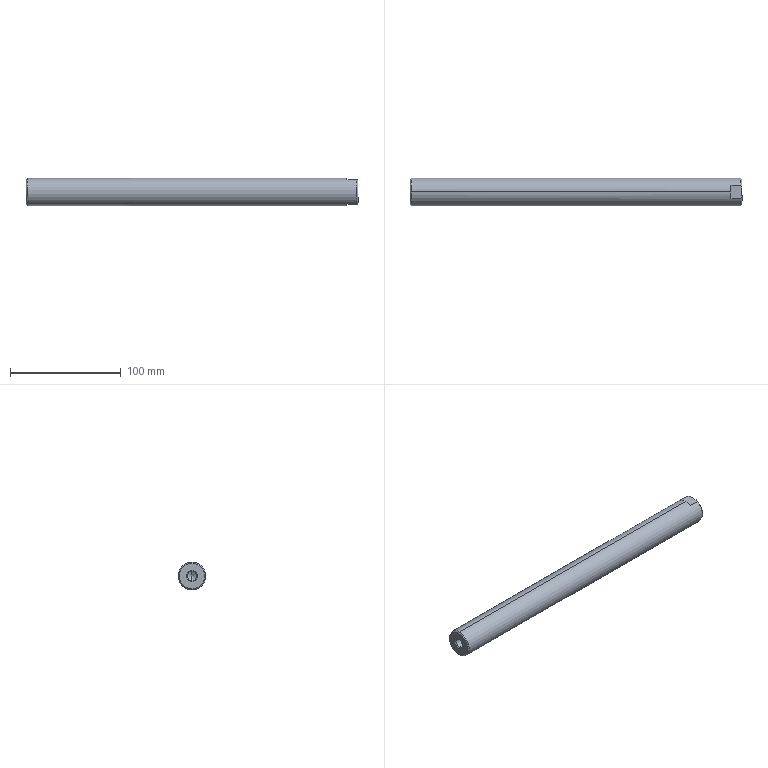Part | STEP file | VFJC25-300-M10-SC290-qwwq-a_2 | 1 solid | 18 faces | box 300 x 25 x 25 mm | volume 145438 mm3 | cone 8 | plane 6 | cylinder 4 | commonest cylinder face diameters 8.376 x2 25 x2
STEP:
#1=CARTESIAN_POINT('',(0.,0.,0.));
#2=DIRECTION('',(0.,0.,1.));
#3=DIRECTION('',(1.,0.,0.));
#4=AXIS2_PLACEMENT_3D('',#1,#2,#3);
#5=CARTESIAN_POINT('',(1.,0.,-12.5));
#6=VERTEX_POINT('',#5);
#7=CARTESIAN_POINT('',(1.,0.,12.5));
#8=VERTEX_POINT('',#7);
#9=CARTESIAN_POINT('',(1.,0.,0.));
#10=DIRECTION('',(1.,0.,0.));
#11=DIRECTION('',(0.,0.,-1.));
#12=AXIS2_PLACEMENT_3D('',#9,#10,#11);
#13=CIRCLE('',#12,12.5);
#14=CARTESIAN_POINT('',(300.,0.,0.));
#15=DIRECTION('',(1.,0.,0.));
#16=DIRECTION('',(0.,0.,-1.));
#17=AXIS2_PLACEMENT_3D('',#14,#15,#16);
#18=CYLINDRICAL_SURFACE('',#17,12.5);
#19=CARTESIAN_POINT('',(0.,-299.));
#20=DIRECTION('',(1.,0.));
#21=VECTOR('',#20,1.);
#22=LINE('',#19,#21);
#23=(GEOMETRIC_REPRESENTATION_CONTEXT(2)PARAMETRIC_REPRESENTATION_CONTEXT()REPRESENTATION_CONTEXT('',''));
#24=DEFINITIONAL_REPRESENTATION('',(#22),#23);
#25=PCURVE('',#18,#24);
#26=CARTESIAN_POINT('',(1.,0.,0.));
#27=DIRECTION('',(1.,0.,0.));
#28=DIRECTION('',(0.,0.,-1.));
#29=AXIS2_PLACEMENT_3D('',#26,#27,#28);
#30=CONICAL_SURFACE('',#29,12.5,0.7854);
#31=CARTESIAN_POINT('',(0.,0.));
#32=DIRECTION('',(1.,0.));
#33=VECTOR('',#32,1.);
#34=LINE('',#31,#33);
#35=(GEOMETRIC_REPRESENTATION_CONTEXT(2)PARAMETRIC_REPRESENTATION_CONTEXT()REPRESENTATION_CONTEXT('',''));
#36=DEFINITIONAL_REPRESENTATION('',(#34),#35);
#37=PCURVE('',#30,#36);
#38=SURFACE_CURVE('',#13,(#25,#37),.PCURVE_S1.);
#39=EDGE_CURVE('',#6,#8,#38,.T.);
#40=ORIENTED_EDGE('',*,*,#39,.T.);
#41=CARTESIAN_POINT('',(290.,0.,12.5));
#42=VERTEX_POINT('',#41);
#43=CARTESIAN_POINT('',(300.,0.,12.5));
#44=DIRECTION('',(1.,0.,0.));
#45=VECTOR('',#44,1.);
#46=LINE('',#43,#45);
#47=CARTESIAN_POINT('',(3.142,0.));
#48=DIRECTION('',(0.,1.));
#49=VECTOR('',#48,1.);
#50=LINE('',#47,#49);
#51=(GEOMETRIC_REPRESENTATION_CONTEXT(2)PARAMETRIC_REPRESENTATION_CONTEXT()REPRESENTATION_CONTEXT('',''));
#52=DEFINITIONAL_REPRESENTATION('',(#50),#51);
#53=PCURVE('',#18,#52);
#54=CARTESIAN_POINT('',(300.,0.,0.));
#55=DIRECTION('',(1.,0.,0.));
#56=DIRECTION('',(0.,0.,-1.));
#57=AXIS2_PLACEMENT_3D('',#54,#55,#56);
#58=CYLINDRICAL_SURFACE('',#57,12.5);
#59=CARTESIAN_POINT('',(3.142,0.));
#60=DIRECTION('',(0.,1.));
#61=VECTOR('',#60,1.);
#62=LINE('',#59,#61);
#63=(GEOMETRIC_REPRESENTATION_CONTEXT(2)PARAMETRIC_REPRESENTATION_CONTEXT()REPRESENTATION_CONTEXT('',''));
#64=DEFINITIONAL_REPRESENTATION('',(#62),#63);
#65=PCURVE('',#58,#64);
#66=SURFACE_CURVE('',#46,(#53,#65),.PCURVE_S1.);
#67=EDGE_CURVE('',#8,#42,#66,.T.);
#68=ORIENTED_EDGE('',*,*,#67,.T.);
#69=CARTESIAN_POINT('',(290.,5.937,11.));
#70=VERTEX_POINT('',#69);
#71=CARTESIAN_POINT('',(290.,0.,0.));
#72=DIRECTION('',(-1.,0.,0.));
#73=DIRECTION('',(0.,0.,-1.));
#74=AXIS2_PLACEMENT_3D('',#71,#72,#73);
#75=CIRCLE('',#74,12.5);
#76=CARTESIAN_POINT('',(6.283,-10.));
#77=DIRECTION('',(-1.,0.));
#78=VECTOR('',#77,1.);
#79=LINE('',#76,#78);
#80=(GEOMETRIC_REPRESENTATION_CONTEXT(2)PARAMETRIC_REPRESENTATION_CONTEXT()REPRESENTATION_CONTEXT('',''));
#81=DEFINITIONAL_REPRESENTATION('',(#79),#80);
#82=PCURVE('',#18,#81);
#83=CARTESIAN_POINT('',(290.,0.,0.));
#84=DIRECTION('',(1.,0.,0.));
#85=DIRECTION('',(0.,0.,-1.));
#86=AXIS2_PLACEMENT_3D('',#83,#84,#85);
#87=PLANE('',#86);
#88=CARTESIAN_POINT('',(12.5,0.));
#89=CARTESIAN_POINT('',(12.5,-21.651));
#90=CARTESIAN_POINT('',(-6.25,-10.825));
#91=CARTESIAN_POINT('',(-25.,0.));
#92=CARTESIAN_POINT('',(-6.25,10.825));
#93=CARTESIAN_POINT('',(12.5,21.651));
#94=CARTESIAN_POINT('',(12.5,0.));
#95=(BOUNDED_CURVE()B_SPLINE_CURVE(2,(#88,#89,#90,#91,#92,#93,#94),.UNSPECIFIED.,.T.,.F.)B_SPLINE_CURVE_WITH_KNOTS((1,2,2,2,2,1),(-2.094,0.,2.094,4.189,6.283,8.378),.UNSPECIFIED.)CURVE()GEOMETRIC_REPRESENTATION_ITEM()RATIONAL_B_SPLINE_CURVE((1.,0.5,1.,0.5,1.,0.5,1.))REPRESENTATION_ITEM(''));
#96=(GEOMETRIC_REPRESENTATION_CONTEXT(2)PARAMETRIC_REPRESENTATION_CONTEXT()REPRESENTATION_CONTEXT('',''));
#97=DEFINITIONAL_REPRESENTATION('',(#95),#96);
#98=PCURVE('',#87,#97);
#99=SURFACE_CURVE('',#75,(#82,#98),.PCURVE_S1.);
#100=EDGE_CURVE('',#42,#70,#99,.T.);
#101=ORIENTED_EDGE('',*,*,#100,.T.);
#102=CARTESIAN_POINT('',(299.,5.937,11.));
#103=VERTEX_POINT('',#102);
#104=CARTESIAN_POINT('',(300.,5.937,11.));
#105=DIRECTION('',(1.,0.,0.));
#106=VECTOR('',#105,1.);
#107=LINE('',#104,#106);
#108=CARTESIAN_POINT('',(2.647,0.));
#109=DIRECTION('',(0.,1.));
#110=VECTOR('',#109,1.);
#111=LINE('',#108,#110);
#112=(GEOMETRIC_REPRESENTATION_CONTEXT(2)PARAMETRIC_REPRESENTATION_CONTEXT()REPRESENTATION_CONTEXT('',''));
#113=DEFINITIONAL_REPRESENTATION('',(#111),#112);
#114=PCURVE('',#18,#113);
#115=CARTESIAN_POINT('',(300.,12.5,11.));
#116=DIRECTION('',(0.,0.,-1.));
#117=DIRECTION('',(-1.,0.,0.));
#118=AXIS2_PLACEMENT_3D('',#115,#116,#117);
#119=PLANE('',#118);
#120=CARTESIAN_POINT('',(0.,-6.563));
#121=DIRECTION('',(-1.,0.));
#122=VECTOR('',#121,1.);
#123=LINE('',#120,#122);
#124=(GEOMETRIC_REPRESENTATION_CONTEXT(2)PARAMETRIC_REPRESENTATION_CONTEXT()REPRESENTATION_CONTEXT('',''));
#125=DEFINITIONAL_REPRESENTATION('',(#123),#124);
#126=PCURVE('',#119,#125);
#127=SURFACE_CURVE('',#107,(#114,#126),.PCURVE_S1.);
#128=EDGE_CURVE('',#70,#103,#127,.T.);
#129=ORIENTED_EDGE('',*,*,#128,.T.);
#130=CARTESIAN_POINT('',(299.,5.937,-11.));
#131=VERTEX_POINT('',#130);
#132=CARTESIAN_POINT('',(299.,0.,0.));
#133=DIRECTION('',(-1.,0.,0.));
#134=DIRECTION('',(0.,0.,-1.));
#135=AXIS2_PLACEMENT_3D('',#132,#133,#134);
#136=CIRCLE('',#135,12.5);
#137=CARTESIAN_POINT('',(6.283,-1.));
#138=DIRECTION('',(-1.,0.));
#139=VECTOR('',#138,1.);
#140=LINE('',#137,#139);
#141=(GEOMETRIC_REPRESENTATION_CONTEXT(2)PARAMETRIC_REPRESENTATION_CONTEXT()REPRESENTATION_CONTEXT('',''));
#142=DEFINITIONAL_REPRESENTATION('',(#140),#141);
#143=PCURVE('',#18,#142);
#144=CARTESIAN_POINT('',(299.,0.,0.));
#145=DIRECTION('',(-1.,0.,0.));
#146=DIRECTION('',(0.,-1.,0.));
#147=AXIS2_PLACEMENT_3D('',#144,#145,#146);
#148=CONICAL_SURFACE('',#147,12.5,0.7854);
#149=CARTESIAN_POINT('',(-1.571,0.));
#150=DIRECTION('',(1.,0.));
#151=VECTOR('',#150,1.);
#152=LINE('',#149,#151);
#153=(GEOMETRIC_REPRESENTATION_CONTEXT(2)PARAMETRIC_REPRESENTATION_CONTEXT()REPRESENTATION_CONTEXT('',''));
#154=DEFINITIONAL_REPRESENTATION('',(#152),#153);
#155=PCURVE('',#148,#154);
#156=SURFACE_CURVE('',#136,(#143,#155),.PCURVE_S1.);
#157=EDGE_CURVE('',#103,#131,#156,.T.);
#158=ORIENTED_EDGE('',*,*,#157,.T.);
#159=CARTESIAN_POINT('',(290.,5.937,-11.));
#160=VERTEX_POINT('',#159);
#161=CARTESIAN_POINT('',(300.,5.937,-11.));
#162=DIRECTION('',(-1.,0.,0.));
#163=VECTOR('',#162,1.);
#164=LINE('',#161,#163);
#165=CARTESIAN_POINT('',(0.4949,0.));
#166=DIRECTION('',(0.,-1.));
#167=VECTOR('',#166,1.);
#168=LINE('',#165,#167);
#169=(GEOMETRIC_REPRESENTATION_CONTEXT(2)PARAMETRIC_REPRESENTATION_CONTEXT()REPRESENTATION_CONTEXT('',''));
#170=DEFINITIONAL_REPRESENTATION('',(#168),#169);
#171=PCURVE('',#18,#170);
#172=CARTESIAN_POINT('',(300.,-12.5,-11.));
#173=DIRECTION('',(0.,0.,1.));
#174=DIRECTION('',(1.,0.,0.));
#175=AXIS2_PLACEMENT_3D('',#172,#173,#174);
#176=PLANE('',#175);
#177=CARTESIAN_POINT('',(0.,18.437));
#178=DIRECTION('',(-1.,0.));
#179=VECTOR('',#178,1.);
#180=LINE('',#177,#179);
#181=(GEOMETRIC_REPRESENTATION_CONTEXT(2)PARAMETRIC_REPRESENTATION_CONTEXT()REPRESENTATION_CONTEXT('',''));
#182=DEFINITIONAL_REPRESENTATION('',(#180),#181);
#183=PCURVE('',#176,#182);
#184=SURFACE_CURVE('',#164,(#171,#183),.PCURVE_S1.);
#185=EDGE_CURVE('',#131,#160,#184,.T.);
#186=ORIENTED_EDGE('',*,*,#185,.T.);
#187=CARTESIAN_POINT('',(290.,0.,-12.5));
#188=VERTEX_POINT('',#187);
#189=CARTESIAN_POINT('',(290.,0.,0.));
#190=DIRECTION('',(-1.,0.,0.));
#191=DIRECTION('',(0.,0.,-1.));
#192=AXIS2_PLACEMENT_3D('',#189,#190,#191);
#193=CIRCLE('',#192,12.5);
#194=CARTESIAN_POINT('',(6.283,-10.));
#195=DIRECTION('',(-1.,0.));
#196=VECTOR('',#195,1.);
#197=LINE('',#194,#196);
#198=(GEOMETRIC_REPRESENTATION_CONTEXT(2)PARAMETRIC_REPRESENTATION_CONTEXT()REPRESENTATION_CONTEXT('',''));
#199=DEFINITIONAL_REPRESENTATION('',(#197),#198);
#200=PCURVE('',#18,#199);
#201=CARTESIAN_POINT('',(290.,0.,0.));
#202=DIRECTION('',(1.,0.,0.));
#203=DIRECTION('',(0.,0.,-1.));
#204=AXIS2_PLACEMENT_3D('',#201,#202,#203);
#205=PLANE('',#204);
#206=CARTESIAN_POINT('',(12.5,0.));
#207=CARTESIAN_POINT('',(12.5,-21.651));
#208=CARTESIAN_POINT('',(-6.25,-10.825));
#209=CARTESIAN_POINT('',(-25.,0.));
#210=CARTESIAN_POINT('',(-6.25,10.825));
#211=CARTESIAN_POINT('',(12.5,21.651));
#212=CARTESIAN_POINT('',(12.5,0.));
#213=(BOUNDED_CURVE()B_SPLINE_CURVE(2,(#206,#207,#208,#209,#210,#211,#212),.UNSPECIFIED.,.T.,.F.)B_SPLINE_CURVE_WITH_KNOTS((1,2,2,2,2,1),(-2.094,0.,2.094,4.189,6.283,8.378),.UNSPECIFIED.)CURVE()GEOMETRIC_REPRESENTATION_ITEM()RATIONAL_B_SPLINE_CURVE((1.,0.5,1.,0.5,1.,0.5,1.))REPRESENTATION_ITEM(''));
#214=(GEOMETRIC_REPRESENTATION_CONTEXT(2)PARAMETRIC_REPRESENTATION_CONTEXT()REPRESENTATION_CONTEXT('',''));
#215=DEFINITIONAL_REPRESENTATION('',(#213),#214);
#216=PCURVE('',#205,#215);
#217=SURFACE_CURVE('',#193,(#200,#216),.PCURVE_S1.);
#218=EDGE_CURVE('',#160,#188,#217,.T.);
#219=ORIENTED_EDGE('',*,*,#218,.T.);
#220=CARTESIAN_POINT('',(300.,0.,-12.5));
#221=DIRECTION('',(1.,0.,0.));
#222=VECTOR('',#221,1.);
#223=LINE('',#220,#222);
#224=CARTESIAN_POINT('',(0.,0.));
#225=DIRECTION('',(0.,1.));
#226=VECTOR('',#225,1.);
#227=LINE('',#224,#226);
#228=(GEOMETRIC_REPRESENTATION_CONTEXT(2)PARAMETRIC_REPRESENTATION_CONTEXT()REPRESENTATION_CONTEXT('',''));
#229=DEFINITIONAL_REPRESENTATION('',(#227),#228);
#230=PCURVE('',#18,#229);
#231=CARTESIAN_POINT('',(6.283,0.));
#232=DIRECTION('',(0.,1.));
#233=VECTOR('',#232,1.);
#234=LINE('',#231,#233);
#235=(GEOMETRIC_REPRESENTATION_CONTEXT(2)PARAMETRIC_REPRESENTATION_CONTEXT()REPRESENTATION_CONTEXT('',''));
#236=DEFINITIONAL_REPRESENTATION('',(#234),#235);
#237=PCURVE('',#58,#236);
#238=SURFACE_CURVE('',#223,(#230,#237),.PCURVE_S1.);
#239=EDGE_CURVE('',#6,#188,#238,.T.);
#240=ORIENTED_EDGE('',*,*,#239,.F.);
#241=EDGE_LOOP('',(#40,#68,#101,#129,#158,#186,#219,#240));
#242=FACE_BOUND('',#241,.T.);
#243=ADVANCED_FACE('',(#242),#18,.T.);
#244=CARTESIAN_POINT('',(0.,0.,-11.5));
#245=VERTEX_POINT('',#244);
#246=CARTESIAN_POINT('',(0.,0.,11.5));
#247=VERTEX_POINT('',#246);
#248=CARTESIAN_POINT('',(0.,0.,0.));
#249=DIRECTION('',(1.,0.,0.));
#250=DIRECTION('',(0.,0.,-1.));
#251=AXIS2_PLACEMENT_3D('',#248,#249,#250);
#252=CIRCLE('',#251,11.5);
#253=CARTESIAN_POINT('',(0.,-1.));
#254=DIRECTION('',(1.,0.));
#255=VECTOR('',#254,1.);
#256=LINE('',#253,#255);
#257=(GEOMETRIC_REPRESENTATION_CONTEXT(2)PARAMETRIC_REPRESENTATION_CONTEXT()REPRESENTATION_CONTEXT('',''));
#258=DEFINITIONAL_REPRESENTATION('',(#256),#257);
#259=PCURVE('',#30,#258);
#260=CARTESIAN_POINT('',(0.,0.,0.));
#261=DIRECTION('',(1.,0.,0.));
#262=DIRECTION('',(0.,0.,-1.));
#263=AXIS2_PLACEMENT_3D('',#260,#261,#262);
#264=PLANE('',#263);
#265=CARTESIAN_POINT('',(0.,0.));
#266=DIRECTION('',(1.,0.));
#267=AXIS2_PLACEMENT_2D('',#265,#266);
#268=CIRCLE('',#267,11.5);
#269=(GEOMETRIC_REPRESENTATION_CONTEXT(2)PARAMETRIC_REPRESENTATION_CONTEXT()REPRESENTATION_CONTEXT('',''));
#270=DEFINITIONAL_REPRESENTATION('',(#268),#269);
#271=PCURVE('',#264,#270);
#272=SURFACE_CURVE('',#252,(#259,#271),.PCURVE_S1.);
#273=EDGE_CURVE('',#245,#247,#272,.T.);
#274=ORIENTED_EDGE('',*,*,#273,.T.);
#275=CARTESIAN_POINT('',(1.,0.,12.5));
#276=DIRECTION('',(0.7071,0.,0.7071));
#277=VECTOR('',#276,1.);
#278=LINE('',#275,#277);
#279=CARTESIAN_POINT('',(3.142,0.));
#280=DIRECTION('',(0.,1.));
#281=VECTOR('',#280,1.);
#282=LINE('',#279,#281);
#283=(GEOMETRIC_REPRESENTATION_CONTEXT(2)PARAMETRIC_REPRESENTATION_CONTEXT()REPRESENTATION_CONTEXT('',''));
#284=DEFINITIONAL_REPRESENTATION('',(#282),#283);
#285=PCURVE('',#30,#284);
#286=CARTESIAN_POINT('',(1.,0.,0.));
#287=DIRECTION('',(1.,0.,0.));
#288=DIRECTION('',(0.,0.,-1.));
#289=AXIS2_PLACEMENT_3D('',#286,#287,#288);
#290=CONICAL_SURFACE('',#289,12.5,0.7854);
#291=CARTESIAN_POINT('',(3.142,0.));
#292=DIRECTION('',(0.,1.));
#293=VECTOR('',#292,1.);
#294=LINE('',#291,#293);
#295=(GEOMETRIC_REPRESENTATION_CONTEXT(2)PARAMETRIC_REPRESENTATION_CONTEXT()REPRESENTATION_CONTEXT('',''));
#296=DEFINITIONAL_REPRESENTATION('',(#294),#295);
#297=PCURVE('',#290,#296);
#298=SURFACE_CURVE('',#278,(#285,#297),.PCURVE_S1.);
#299=EDGE_CURVE('',#247,#8,#298,.T.);
#300=ORIENTED_EDGE('',*,*,#299,.T.);
#301=ORIENTED_EDGE('',*,*,#39,.F.);
#302=CARTESIAN_POINT('',(1.,0.,-12.5));
#303=DIRECTION('',(0.7071,0.,-0.7071));
#304=VECTOR('',#303,1.);
#305=LINE('',#302,#304);
#306=CARTESIAN_POINT('',(0.,0.));
#307=DIRECTION('',(0.,1.));
#308=VECTOR('',#307,1.);
#309=LINE('',#306,#308);
#310=(GEOMETRIC_REPRESENTATION_CONTEXT(2)PARAMETRIC_REPRESENTATION_CONTEXT()REPRESENTATION_CONTEXT('',''));
#311=DEFINITIONAL_REPRESENTATION('',(#309),#310);
#312=PCURVE('',#30,#311);
#313=CARTESIAN_POINT('',(6.283,0.));
#314=DIRECTION('',(0.,1.));
#315=VECTOR('',#314,1.);
#316=LINE('',#313,#315);
#317=(GEOMETRIC_REPRESENTATION_CONTEXT(2)PARAMETRIC_REPRESENTATION_CONTEXT()REPRESENTATION_CONTEXT('',''));
#318=DEFINITIONAL_REPRESENTATION('',(#316),#317);
#319=PCURVE('',#290,#318);
#320=SURFACE_CURVE('',#305,(#312,#319),.PCURVE_S1.);
#321=EDGE_CURVE('',#245,#6,#320,.T.);
#322=ORIENTED_EDGE('',*,*,#321,.F.);
#323=EDGE_LOOP('',(#274,#300,#301,#322));
#324=FACE_BOUND('',#323,.T.);
#325=ADVANCED_FACE('',(#324),#30,.T.);
#326=CARTESIAN_POINT('',(0.812,0.,4.188));
#327=VERTEX_POINT('',#326);
#328=CARTESIAN_POINT('',(0.,0.,5.));
#329=VERTEX_POINT('',#328);
#330=CARTESIAN_POINT('',(0.,0.,5.));
#331=DIRECTION('',(-0.7071,0.,0.7071));
#332=VECTOR('',#331,1.);
#333=LINE('',#330,#332);
#334=CARTESIAN_POINT('',(0.,0.,0.));
#335=DIRECTION('',(-1.,0.,0.));
#336=DIRECTION('',(0.,0.,1.));
#337=AXIS2_PLACEMENT_3D('',#334,#335,#336);
#338=CONICAL_SURFACE('',#337,5.,0.7854);
#339=CARTESIAN_POINT('',(6.283,0.));
#340=DIRECTION('',(0.,1.));
#341=VECTOR('',#340,1.);
#342=LINE('',#339,#341);
#343=(GEOMETRIC_REPRESENTATION_CONTEXT(2)PARAMETRIC_REPRESENTATION_CONTEXT()REPRESENTATION_CONTEXT('',''));
#344=DEFINITIONAL_REPRESENTATION('',(#342),#343);
#345=PCURVE('',#338,#344);
#346=CARTESIAN_POINT('',(0.,0.,0.));
#347=DIRECTION('',(-1.,0.,0.));
#348=DIRECTION('',(0.,0.,1.));
#349=AXIS2_PLACEMENT_3D('',#346,#347,#348);
#350=CONICAL_SURFACE('',#349,5.,0.7854);
#351=CARTESIAN_POINT('',(0.,0.));
#352=DIRECTION('',(0.,1.));
#353=VECTOR('',#352,1.);
#354=LINE('',#351,#353);
#355=(GEOMETRIC_REPRESENTATION_CONTEXT(2)PARAMETRIC_REPRESENTATION_CONTEXT()REPRESENTATION_CONTEXT('',''));
#356=DEFINITIONAL_REPRESENTATION('',(#354),#355);
#357=PCURVE('',#350,#356);
#358=SURFACE_CURVE('',#333,(#345,#357),.PCURVE_S1.);
#359=EDGE_CURVE('',#327,#329,#358,.T.);
#360=ORIENTED_EDGE('',*,*,#359,.T.);
#361=CARTESIAN_POINT('',(0.,0.,-5.));
#362=VERTEX_POINT('',#361);
#363=CARTESIAN_POINT('',(0.,0.,0.));
#364=DIRECTION('',(-1.,0.,0.));
#365=DIRECTION('',(0.,0.,1.));
#366=AXIS2_PLACEMENT_3D('',#363,#364,#365);
#367=CIRCLE('',#366,5.);
#368=CARTESIAN_POINT('',(0.,0.));
#369=DIRECTION('',(1.,0.));
#370=VECTOR('',#369,1.);
#371=LINE('',#368,#370);
#372=(GEOMETRIC_REPRESENTATION_CONTEXT(2)PARAMETRIC_REPRESENTATION_CONTEXT()REPRESENTATION_CONTEXT('',''));
#373=DEFINITIONAL_REPRESENTATION('',(#371),#372);
#374=PCURVE('',#338,#373);
#375=CARTESIAN_POINT('',(-5.,0.));
#376=CARTESIAN_POINT('',(-5.,8.66));
#377=CARTESIAN_POINT('',(2.5,4.33));
#378=CARTESIAN_POINT('',(10.,0.));
#379=CARTESIAN_POINT('',(2.5,-4.33));
#380=CARTESIAN_POINT('',(-5.,-8.66));
#381=CARTESIAN_POINT('',(-5.,0.));
#382=(BOUNDED_CURVE()B_SPLINE_CURVE(2,(#375,#376,#377,#378,#379,#380,#381),.UNSPECIFIED.,.T.,.F.)B_SPLINE_CURVE_WITH_KNOTS((1,2,2,2,2,1),(-2.094,0.,2.094,4.189,6.283,8.378),.UNSPECIFIED.)CURVE()GEOMETRIC_REPRESENTATION_ITEM()RATIONAL_B_SPLINE_CURVE((1.,0.5,1.,0.5,1.,0.5,1.))REPRESENTATION_ITEM(''));
#383=(GEOMETRIC_REPRESENTATION_CONTEXT(2)PARAMETRIC_REPRESENTATION_CONTEXT()REPRESENTATION_CONTEXT('',''));
#384=DEFINITIONAL_REPRESENTATION('',(#382),#383);
#385=PCURVE('',#264,#384);
#386=SURFACE_CURVE('',#367,(#374,#385),.PCURVE_S1.);
#387=EDGE_CURVE('',#362,#329,#386,.T.);
#388=ORIENTED_EDGE('',*,*,#387,.F.);
#389=CARTESIAN_POINT('',(0.812,0.,-4.188));
#390=VERTEX_POINT('',#389);
#391=CARTESIAN_POINT('',(0.,0.,-5.));
#392=DIRECTION('',(-0.7071,0.,-0.7071));
#393=VECTOR('',#392,1.);
#394=LINE('',#391,#393);
#395=CARTESIAN_POINT('',(3.142,0.));
#396=DIRECTION('',(0.,1.));
#397=VECTOR('',#396,1.);
#398=LINE('',#395,#397);
#399=(GEOMETRIC_REPRESENTATION_CONTEXT(2)PARAMETRIC_REPRESENTATION_CONTEXT()REPRESENTATION_CONTEXT('',''));
#400=DEFINITIONAL_REPRESENTATION('',(#398),#399);
#401=PCURVE('',#338,#400);
#402=CARTESIAN_POINT('',(3.142,0.));
#403=DIRECTION('',(0.,1.));
#404=VECTOR('',#403,1.);
#405=LINE('',#402,#404);
#406=(GEOMETRIC_REPRESENTATION_CONTEXT(2)PARAMETRIC_REPRESENTATION_CONTEXT()REPRESENTATION_CONTEXT('',''));
#407=DEFINITIONAL_REPRESENTATION('',(#405),#406);
#408=PCURVE('',#350,#407);
#409=SURFACE_CURVE('',#394,(#401,#408),.PCURVE_S1.);
#410=EDGE_CURVE('',#390,#362,#409,.T.);
#411=ORIENTED_EDGE('',*,*,#410,.F.);
#412=CARTESIAN_POINT('',(0.812,0.,0.));
#413=DIRECTION('',(-1.,0.,0.));
#414=DIRECTION('',(0.,0.,1.));
#415=AXIS2_PLACEMENT_3D('',#412,#413,#414);
#416=CIRCLE('',#415,4.188);
#417=CARTESIAN_POINT('',(0.,-0.812));
#418=DIRECTION('',(1.,0.));
#419=VECTOR('',#418,1.);
#420=LINE('',#417,#419);
#421=(GEOMETRIC_REPRESENTATION_CONTEXT(2)PARAMETRIC_REPRESENTATION_CONTEXT()REPRESENTATION_CONTEXT('',''));
#422=DEFINITIONAL_REPRESENTATION('',(#420),#421);
#423=PCURVE('',#338,#422);
#424=CARTESIAN_POINT('',(29.,0.,0.));
#425=DIRECTION('',(1.,0.,0.));
#426=DIRECTION('',(0.,0.,-1.));
#427=AXIS2_PLACEMENT_3D('',#424,#425,#426);
#428=CYLINDRICAL_SURFACE('',#427,4.188);
#429=CARTESIAN_POINT('',(9.425,-28.188));
#430=DIRECTION('',(-1.,0.));
#431=VECTOR('',#430,1.);
#432=LINE('',#429,#431);
#433=(GEOMETRIC_REPRESENTATION_CONTEXT(2)PARAMETRIC_REPRESENTATION_CONTEXT()REPRESENTATION_CONTEXT('',''));
#434=DEFINITIONAL_REPRESENTATION('',(#432),#433);
#435=PCURVE('',#428,#434);
#436=SURFACE_CURVE('',#416,(#423,#435),.PCURVE_S1.);
#437=EDGE_CURVE('',#390,#327,#436,.T.);
#438=ORIENTED_EDGE('',*,*,#437,.T.);
#439=EDGE_LOOP('',(#360,#388,#411,#438));
#440=FACE_BOUND('',#439,.F.);
#441=ADVANCED_FACE('',(#440),#338,.F.);
#442=CARTESIAN_POINT('',(26.582,0.,-4.188));
#443=VERTEX_POINT('',#442);
#444=CARTESIAN_POINT('',(29.,0.,-4.188));
#445=DIRECTION('',(1.,0.,0.));
#446=VECTOR('',#445,1.);
#447=LINE('',#444,#446);
#448=CARTESIAN_POINT('',(6.283,0.));
#449=DIRECTION('',(0.,1.));
#450=VECTOR('',#449,1.);
#451=LINE('',#448,#450);
#452=(GEOMETRIC_REPRESENTATION_CONTEXT(2)PARAMETRIC_REPRESENTATION_CONTEXT()REPRESENTATION_CONTEXT('',''));
#453=DEFINITIONAL_REPRESENTATION('',(#451),#452);
#454=PCURVE('',#428,#453);
#455=CARTESIAN_POINT('',(29.,0.,0.));
#456=DIRECTION('',(1.,0.,0.));
#457=DIRECTION('',(0.,0.,-1.));
#458=AXIS2_PLACEMENT_3D('',#455,#456,#457);
#459=CYLINDRICAL_SURFACE('',#458,4.188);
#460=CARTESIAN_POINT('',(0.,0.));
#461=DIRECTION('',(0.,1.));
#462=VECTOR('',#461,1.);
#463=LINE('',#460,#462);
#464=(GEOMETRIC_REPRESENTATION_CONTEXT(2)PARAMETRIC_REPRESENTATION_CONTEXT()REPRESENTATION_CONTEXT('',''));
#465=DEFINITIONAL_REPRESENTATION('',(#463),#464);
#466=PCURVE('',#459,#465);
#467=SURFACE_CURVE('',#447,(#454,#466),.PCURVE_S1.);
#468=EDGE_CURVE('',#390,#443,#467,.T.);
#469=ORIENTED_EDGE('',*,*,#468,.T.);
#470=CARTESIAN_POINT('',(26.582,0.,4.188));
#471=VERTEX_POINT('',#470);
#472=CARTESIAN_POINT('',(26.582,0.,0.));
#473=DIRECTION('',(-1.,0.,0.));
#474=DIRECTION('',(0.,0.,-1.));
#475=AXIS2_PLACEMENT_3D('',#472,#473,#474);
#476=CIRCLE('',#475,4.188);
#477=CARTESIAN_POINT('',(6.283,-2.418));
#478=DIRECTION('',(-1.,0.));
#479=VECTOR('',#478,1.);
#480=LINE('',#477,#479);
#481=(GEOMETRIC_REPRESENTATION_CONTEXT(2)PARAMETRIC_REPRESENTATION_CONTEXT()REPRESENTATION_CONTEXT('',''));
#482=DEFINITIONAL_REPRESENTATION('',(#480),#481);
#483=PCURVE('',#428,#482);
#484=CARTESIAN_POINT('',(26.582,0.,0.));
#485=DIRECTION('',(-1.,0.,0.));
#486=DIRECTION('',(0.,0.,1.));
#487=AXIS2_PLACEMENT_3D('',#484,#485,#486);
#488=CONICAL_SURFACE('',#487,4.188,1.047);
#489=CARTESIAN_POINT('',(3.142,0.));
#490=DIRECTION('',(1.,0.));
#491=VECTOR('',#490,1.);
#492=LINE('',#489,#491);
#493=(GEOMETRIC_REPRESENTATION_CONTEXT(2)PARAMETRIC_REPRESENTATION_CONTEXT()REPRESENTATION_CONTEXT('',''));
#494=DEFINITIONAL_REPRESENTATION('',(#492),#493);
#495=PCURVE('',#488,#494);
#496=SURFACE_CURVE('',#476,(#483,#495),.PCURVE_S1.);
#497=EDGE_CURVE('',#443,#471,#496,.T.);
#498=ORIENTED_EDGE('',*,*,#497,.T.);
#499=CARTESIAN_POINT('',(29.,0.,4.188));
#500=DIRECTION('',(1.,0.,0.));
#501=VECTOR('',#500,1.);
#502=LINE('',#499,#501);
#503=CARTESIAN_POINT('',(3.142,0.));
#504=DIRECTION('',(0.,1.));
#505=VECTOR('',#504,1.);
#506=LINE('',#503,#505);
#507=(GEOMETRIC_REPRESENTATION_CONTEXT(2)PARAMETRIC_REPRESENTATION_CONTEXT()REPRESENTATION_CONTEXT('',''));
#508=DEFINITIONAL_REPRESENTATION('',(#506),#507);
#509=PCURVE('',#428,#508);
#510=CARTESIAN_POINT('',(3.142,0.));
#511=DIRECTION('',(0.,1.));
#512=VECTOR('',#511,1.);
#513=LINE('',#510,#512);
#514=(GEOMETRIC_REPRESENTATION_CONTEXT(2)PARAMETRIC_REPRESENTATION_CONTEXT()REPRESENTATION_CONTEXT('',''));
#515=DEFINITIONAL_REPRESENTATION('',(#513),#514);
#516=PCURVE('',#459,#515);
#517=SURFACE_CURVE('',#502,(#509,#516),.PCURVE_S1.);
#518=EDGE_CURVE('',#327,#471,#517,.T.);
#519=ORIENTED_EDGE('',*,*,#518,.F.);
#520=ORIENTED_EDGE('',*,*,#437,.F.);
#521=EDGE_LOOP('',(#469,#498,#519,#520));
#522=FACE_BOUND('',#521,.F.);
#523=ADVANCED_FACE('',(#522),#428,.F.);
#524=ORIENTED_EDGE('',*,*,#497,.F.);
#525=CARTESIAN_POINT('',(29.,0.,0.));
#526=VERTEX_POINT('',#525);
#527=CARTESIAN_POINT('',(26.582,0.,-4.188));
#528=DIRECTION('',(-0.5,0.,-0.866));
#529=VECTOR('',#528,1.);
#530=LINE('',#527,#529);
#531=CARTESIAN_POINT('',(3.142,0.));
#532=DIRECTION('',(0.,1.));
#533=VECTOR('',#532,1.);
#534=LINE('',#531,#533);
#535=(GEOMETRIC_REPRESENTATION_CONTEXT(2)PARAMETRIC_REPRESENTATION_CONTEXT()REPRESENTATION_CONTEXT('',''));
#536=DEFINITIONAL_REPRESENTATION('',(#534),#535);
#537=PCURVE('',#488,#536);
#538=CARTESIAN_POINT('',(26.582,0.,0.));
#539=DIRECTION('',(-1.,0.,0.));
#540=DIRECTION('',(0.,0.,1.));
#541=AXIS2_PLACEMENT_3D('',#538,#539,#540);
#542=CONICAL_SURFACE('',#541,4.188,1.047);
#543=CARTESIAN_POINT('',(3.142,0.));
#544=DIRECTION('',(0.,1.));
#545=VECTOR('',#544,1.);
#546=LINE('',#543,#545);
#547=(GEOMETRIC_REPRESENTATION_CONTEXT(2)PARAMETRIC_REPRESENTATION_CONTEXT()REPRESENTATION_CONTEXT('',''));
#548=DEFINITIONAL_REPRESENTATION('',(#546),#547);
#549=PCURVE('',#542,#548);
#550=SURFACE_CURVE('',#530,(#537,#549),.PCURVE_S1.);
#551=EDGE_CURVE('',#526,#443,#550,.T.);
#552=ORIENTED_EDGE('',*,*,#551,.F.);
#553=CARTESIAN_POINT('',(26.582,0.,4.188));
#554=DIRECTION('',(-0.5,0.,0.866));
#555=VECTOR('',#554,1.);
#556=LINE('',#553,#555);
#557=CARTESIAN_POINT('',(6.283,0.));
#558=DIRECTION('',(0.,1.));
#559=VECTOR('',#558,1.);
#560=LINE('',#557,#559);
#561=(GEOMETRIC_REPRESENTATION_CONTEXT(2)PARAMETRIC_REPRESENTATION_CONTEXT()REPRESENTATION_CONTEXT('',''));
#562=DEFINITIONAL_REPRESENTATION('',(#560),#561);
#563=PCURVE('',#488,#562);
#564=CARTESIAN_POINT('',(0.,0.));
#565=DIRECTION('',(0.,1.));
#566=VECTOR('',#565,1.);
#567=LINE('',#564,#566);
#568=(GEOMETRIC_REPRESENTATION_CONTEXT(2)PARAMETRIC_REPRESENTATION_CONTEXT()REPRESENTATION_CONTEXT('',''));
#569=DEFINITIONAL_REPRESENTATION('',(#567),#568);
#570=PCURVE('',#542,#569);
#571=SURFACE_CURVE('',#556,(#563,#570),.PCURVE_S1.);
#572=EDGE_CURVE('',#526,#471,#571,.T.);
#573=ORIENTED_EDGE('',*,*,#572,.T.);
#574=EDGE_LOOP('',(#524,#552,#573));
#575=FACE_BOUND('',#574,.F.);
#576=ADVANCED_FACE('',(#575),#488,.F.);
#577=ORIENTED_EDGE('',*,*,#67,.F.);
#578=CARTESIAN_POINT('',(1.,0.,0.));
#579=DIRECTION('',(1.,0.,0.));
#580=DIRECTION('',(0.,0.,-1.));
#581=AXIS2_PLACEMENT_3D('',#578,#579,#580);
#582=CIRCLE('',#581,12.5);
#583=CARTESIAN_POINT('',(0.,-299.));
#584=DIRECTION('',(1.,0.));
#585=VECTOR('',#584,1.);
#586=LINE('',#583,#585);
#587=(GEOMETRIC_REPRESENTATION_CONTEXT(2)PARAMETRIC_REPRESENTATION_CONTEXT()REPRESENTATION_CONTEXT('',''));
#588=DEFINITIONAL_REPRESENTATION('',(#586),#587);
#589=PCURVE('',#58,#588);
#590=CARTESIAN_POINT('',(0.,0.));
#591=DIRECTION('',(1.,0.));
#592=VECTOR('',#591,1.);
#593=LINE('',#590,#592);
#594=(GEOMETRIC_REPRESENTATION_CONTEXT(2)PARAMETRIC_REPRESENTATION_CONTEXT()REPRESENTATION_CONTEXT('',''));
#595=DEFINITIONAL_REPRESENTATION('',(#593),#594);
#596=PCURVE('',#290,#595);
#597=SURFACE_CURVE('',#582,(#589,#596),.PCURVE_S1.);
#598=EDGE_CURVE('',#8,#6,#597,.T.);
#599=ORIENTED_EDGE('',*,*,#598,.T.);
#600=ORIENTED_EDGE('',*,*,#239,.T.);
#601=CARTESIAN_POINT('',(290.,-5.937,-11.));
#602=VERTEX_POINT('',#601);
#603=CARTESIAN_POINT('',(290.,0.,0.));
#604=DIRECTION('',(-1.,0.,0.));
#605=DIRECTION('',(0.,0.,-1.));
#606=AXIS2_PLACEMENT_3D('',#603,#604,#605);
#607=CIRCLE('',#606,12.5);
#608=CARTESIAN_POINT('',(6.283,-10.));
#609=DIRECTION('',(-1.,0.));
#610=VECTOR('',#609,1.);
#611=LINE('',#608,#610);
#612=(GEOMETRIC_REPRESENTATION_CONTEXT(2)PARAMETRIC_REPRESENTATION_CONTEXT()REPRESENTATION_CONTEXT('',''));
#613=DEFINITIONAL_REPRESENTATION('',(#611),#612);
#614=PCURVE('',#58,#613);
#615=CARTESIAN_POINT('',(12.5,0.));
#616=CARTESIAN_POINT('',(12.5,-21.651));
#617=CARTESIAN_POINT('',(-6.25,-10.825));
#618=CARTESIAN_POINT('',(-25.,0.));
#619=CARTESIAN_POINT('',(-6.25,10.825));
#620=CARTESIAN_POINT('',(12.5,21.651));
#621=CARTESIAN_POINT('',(12.5,0.));
#622=(BOUNDED_CURVE()B_SPLINE_CURVE(2,(#615,#616,#617,#618,#619,#620,#621),.UNSPECIFIED.,.T.,.F.)B_SPLINE_CURVE_WITH_KNOTS((1,2,2,2,2,1),(-2.094,0.,2.094,4.189,6.283,8.378),.UNSPECIFIED.)CURVE()GEOMETRIC_REPRESENTATION_ITEM()RATIONAL_B_SPLINE_CURVE((1.,0.5,1.,0.5,1.,0.5,1.))REPRESENTATION_ITEM(''));
#623=(GEOMETRIC_REPRESENTATION_CONTEXT(2)PARAMETRIC_REPRESENTATION_CONTEXT()REPRESENTATION_CONTEXT('',''));
#624=DEFINITIONAL_REPRESENTATION('',(#622),#623);
#625=PCURVE('',#205,#624);
#626=SURFACE_CURVE('',#607,(#614,#625),.PCURVE_S1.);
#627=EDGE_CURVE('',#188,#602,#626,.T.);
#628=ORIENTED_EDGE('',*,*,#627,.T.);
#629=CARTESIAN_POINT('',(299.,-5.937,-11.));
#630=VERTEX_POINT('',#629);
#631=CARTESIAN_POINT('',(300.,-5.937,-11.));
#632=DIRECTION('',(1.,0.,0.));
#633=VECTOR('',#632,1.);
#634=LINE('',#631,#633);
#635=CARTESIAN_POINT('',(5.788,0.));
#636=DIRECTION('',(0.,1.));
#637=VECTOR('',#636,1.);
#638=LINE('',#635,#637);
#639=(GEOMETRIC_REPRESENTATION_CONTEXT(2)PARAMETRIC_REPRESENTATION_CONTEXT()REPRESENTATION_CONTEXT('',''));
#640=DEFINITIONAL_REPRESENTATION('',(#638),#639);
#641=PCURVE('',#58,#640);
#642=CARTESIAN_POINT('',(0.,6.563));
#643=DIRECTION('',(1.,0.));
#644=VECTOR('',#643,1.);
#645=LINE('',#642,#644);
#646=(GEOMETRIC_REPRESENTATION_CONTEXT(2)PARAMETRIC_REPRESENTATION_CONTEXT()REPRESENTATION_CONTEXT('',''));
#647=DEFINITIONAL_REPRESENTATION('',(#645),#646);
#648=PCURVE('',#176,#647);
#649=SURFACE_CURVE('',#634,(#641,#648),.PCURVE_S1.);
#650=EDGE_CURVE('',#602,#630,#649,.T.);
#651=ORIENTED_EDGE('',*,*,#650,.T.);
#652=CARTESIAN_POINT('',(299.,-5.937,11.));
#653=VERTEX_POINT('',#652);
#654=CARTESIAN_POINT('',(299.,0.,0.));
#655=DIRECTION('',(-1.,0.,0.));
#656=DIRECTION('',(0.,0.,-1.));
#657=AXIS2_PLACEMENT_3D('',#654,#655,#656);
#658=CIRCLE('',#657,12.5);
#659=CARTESIAN_POINT('',(6.283,-1.));
#660=DIRECTION('',(-1.,0.));
#661=VECTOR('',#660,1.);
#662=LINE('',#659,#661);
#663=(GEOMETRIC_REPRESENTATION_CONTEXT(2)PARAMETRIC_REPRESENTATION_CONTEXT()REPRESENTATION_CONTEXT('',''));
#664=DEFINITIONAL_REPRESENTATION('',(#662),#663);
#665=PCURVE('',#58,#664);
#666=CARTESIAN_POINT('',(299.,0.,0.));
#667=DIRECTION('',(-1.,0.,0.));
#668=DIRECTION('',(0.,0.,1.));
#669=AXIS2_PLACEMENT_3D('',#666,#667,#668);
#670=CONICAL_SURFACE('',#669,12.5,0.7854);
#671=CARTESIAN_POINT('',(3.142,0.));
#672=DIRECTION('',(1.,0.));
#673=VECTOR('',#672,1.);
#674=LINE('',#671,#673);
#675=(GEOMETRIC_REPRESENTATION_CONTEXT(2)PARAMETRIC_REPRESENTATION_CONTEXT()REPRESENTATION_CONTEXT('',''));
#676=DEFINITIONAL_REPRESENTATION('',(#674),#675);
#677=PCURVE('',#670,#676);
#678=SURFACE_CURVE('',#658,(#665,#677),.PCURVE_S1.);
#679=EDGE_CURVE('',#630,#653,#678,.T.);
#680=ORIENTED_EDGE('',*,*,#679,.T.);
#681=CARTESIAN_POINT('',(290.,-5.937,11.));
#682=VERTEX_POINT('',#681);
#683=CARTESIAN_POINT('',(300.,-5.937,11.));
#684=DIRECTION('',(-1.,0.,0.));
#685=VECTOR('',#684,1.);
#686=LINE('',#683,#685);
#687=CARTESIAN_POINT('',(3.637,0.));
#688=DIRECTION('',(0.,-1.));
#689=VECTOR('',#688,1.);
#690=LINE('',#687,#689);
#691=(GEOMETRIC_REPRESENTATION_CONTEXT(2)PARAMETRIC_REPRESENTATION_CONTEXT()REPRESENTATION_CONTEXT('',''));
#692=DEFINITIONAL_REPRESENTATION('',(#690),#691);
#693=PCURVE('',#58,#692);
#694=CARTESIAN_POINT('',(0.,-18.437));
#695=DIRECTION('',(1.,0.));
#696=VECTOR('',#695,1.);
#697=LINE('',#694,#696);
#698=(GEOMETRIC_REPRESENTATION_CONTEXT(2)PARAMETRIC_REPRESENTATION_CONTEXT()REPRESENTATION_CONTEXT('',''));
#699=DEFINITIONAL_REPRESENTATION('',(#697),#698);
#700=PCURVE('',#119,#699);
#701=SURFACE_CURVE('',#686,(#693,#700),.PCURVE_S1.);
#702=EDGE_CURVE('',#653,#682,#701,.T.);
#703=ORIENTED_EDGE('',*,*,#702,.T.);
#704=CARTESIAN_POINT('',(290.,0.,0.));
#705=DIRECTION('',(-1.,0.,0.));
#706=DIRECTION('',(0.,0.,-1.));
#707=AXIS2_PLACEMENT_3D('',#704,#705,#706);
#708=CIRCLE('',#707,12.5);
#709=CARTESIAN_POINT('',(6.283,-10.));
#710=DIRECTION('',(-1.,0.));
#711=VECTOR('',#710,1.);
#712=LINE('',#709,#711);
#713=(GEOMETRIC_REPRESENTATION_CONTEXT(2)PARAMETRIC_REPRESENTATION_CONTEXT()REPRESENTATION_CONTEXT('',''));
#714=DEFINITIONAL_REPRESENTATION('',(#712),#713);
#715=PCURVE('',#58,#714);
#716=CARTESIAN_POINT('',(12.5,0.));
#717=CARTESIAN_POINT('',(12.5,-21.651));
#718=CARTESIAN_POINT('',(-6.25,-10.825));
#719=CARTESIAN_POINT('',(-25.,0.));
#720=CARTESIAN_POINT('',(-6.25,10.825));
#721=CARTESIAN_POINT('',(12.5,21.651));
#722=CARTESIAN_POINT('',(12.5,0.));
#723=(BOUNDED_CURVE()B_SPLINE_CURVE(2,(#716,#717,#718,#719,#720,#721,#722),.UNSPECIFIED.,.T.,.F.)B_SPLINE_CURVE_WITH_KNOTS((1,2,2,2,2,1),(-2.094,0.,2.094,4.189,6.283,8.378),.UNSPECIFIED.)CURVE()GEOMETRIC_REPRESENTATION_ITEM()RATIONAL_B_SPLINE_CURVE((1.,0.5,1.,0.5,1.,0.5,1.))REPRESENTATION_ITEM(''));
#724=(GEOMETRIC_REPRESENTATION_CONTEXT(2)PARAMETRIC_REPRESENTATION_CONTEXT()REPRESENTATION_CONTEXT('',''));
#725=DEFINITIONAL_REPRESENTATION('',(#723),#724);
#726=PCURVE('',#87,#725);
#727=SURFACE_CURVE('',#708,(#715,#726),.PCURVE_S1.);
#728=EDGE_CURVE('',#682,#42,#727,.T.);
#729=ORIENTED_EDGE('',*,*,#728,.T.);
#730=EDGE_LOOP('',(#577,#599,#600,#628,#651,#680,#703,#729));
#731=FACE_BOUND('',#730,.T.);
#732=ADVANCED_FACE('',(#731),#58,.T.);
#733=ORIENTED_EDGE('',*,*,#299,.F.);
#734=CARTESIAN_POINT('',(0.,0.,0.));
#735=DIRECTION('',(1.,0.,0.));
#736=DIRECTION('',(0.,0.,-1.));
#737=AXIS2_PLACEMENT_3D('',#734,#735,#736);
#738=CIRCLE('',#737,11.5);
#739=CARTESIAN_POINT('',(0.,-1.));
#740=DIRECTION('',(1.,0.));
#741=VECTOR('',#740,1.);
#742=LINE('',#739,#741);
#743=(GEOMETRIC_REPRESENTATION_CONTEXT(2)PARAMETRIC_REPRESENTATION_CONTEXT()REPRESENTATION_CONTEXT('',''));
#744=DEFINITIONAL_REPRESENTATION('',(#742),#743);
#745=PCURVE('',#290,#744);
#746=CARTESIAN_POINT('',(0.,0.));
#747=DIRECTION('',(1.,0.));
#748=AXIS2_PLACEMENT_2D('',#746,#747);
#749=CIRCLE('',#748,11.5);
#750=(GEOMETRIC_REPRESENTATION_CONTEXT(2)PARAMETRIC_REPRESENTATION_CONTEXT()REPRESENTATION_CONTEXT('',''));
#751=DEFINITIONAL_REPRESENTATION('',(#749),#750);
#752=PCURVE('',#264,#751);
#753=SURFACE_CURVE('',#738,(#745,#752),.PCURVE_S1.);
#754=EDGE_CURVE('',#247,#245,#753,.T.);
#755=ORIENTED_EDGE('',*,*,#754,.T.);
#756=ORIENTED_EDGE('',*,*,#321,.T.);
#757=ORIENTED_EDGE('',*,*,#598,.F.);
#758=EDGE_LOOP('',(#733,#755,#756,#757));
#759=FACE_BOUND('',#758,.T.);
#760=ADVANCED_FACE('',(#759),#290,.T.);
#761=CARTESIAN_POINT('',(290.,0.,-11.));
#762=DIRECTION('',(0.,-1.,0.));
#763=VECTOR('',#762,1.);
#764=LINE('',#761,#763);
#765=CARTESIAN_POINT('',(11.,0.));
#766=DIRECTION('',(0.,-1.));
#767=VECTOR('',#766,1.);
#768=LINE('',#765,#767);
#769=(GEOMETRIC_REPRESENTATION_CONTEXT(2)PARAMETRIC_REPRESENTATION_CONTEXT()REPRESENTATION_CONTEXT('',''));
#770=DEFINITIONAL_REPRESENTATION('',(#768),#769);
#771=PCURVE('',#205,#770);
#772=CARTESIAN_POINT('',(-10.,12.5));
#773=DIRECTION('',(0.,-1.));
#774=VECTOR('',#773,1.);
#775=LINE('',#772,#774);
#776=(GEOMETRIC_REPRESENTATION_CONTEXT(2)PARAMETRIC_REPRESENTATION_CONTEXT()REPRESENTATION_CONTEXT('',''));
#777=DEFINITIONAL_REPRESENTATION('',(#775),#776);
#778=PCURVE('',#176,#777);
#779=SURFACE_CURVE('',#764,(#771,#778),.PCURVE_S1.);
#780=EDGE_CURVE('',#160,#602,#779,.T.);
#781=ORIENTED_EDGE('',*,*,#780,.T.);
#782=ORIENTED_EDGE('',*,*,#627,.F.);
#783=ORIENTED_EDGE('',*,*,#218,.F.);
#784=EDGE_LOOP('',(#781,#782,#783));
#785=FACE_BOUND('',#784,.T.);
#786=ADVANCED_FACE('',(#785),#205,.T.);
#787=CARTESIAN_POINT('',(300.,-3.354,-11.));
#788=VERTEX_POINT('',#787);
#789=CARTESIAN_POINT('',(300.,3.354,-11.));
#790=VERTEX_POINT('',#789);
#791=CARTESIAN_POINT('',(300.,-12.5,-11.));
#792=DIRECTION('',(0.,1.,0.));
#793=VECTOR('',#792,1.);
#794=LINE('',#791,#793);
#795=CARTESIAN_POINT('',(0.,0.));
#796=DIRECTION('',(0.,1.));
#797=VECTOR('',#796,1.);
#798=LINE('',#795,#797);
#799=(GEOMETRIC_REPRESENTATION_CONTEXT(2)PARAMETRIC_REPRESENTATION_CONTEXT()REPRESENTATION_CONTEXT('',''));
#800=DEFINITIONAL_REPRESENTATION('',(#798),#799);
#801=PCURVE('',#176,#800);
#802=CARTESIAN_POINT('',(300.,11.5,0.));
#803=DIRECTION('',(-1.,0.,0.));
#804=DIRECTION('',(0.,0.,1.));
#805=AXIS2_PLACEMENT_3D('',#802,#803,#804);
#806=PLANE('',#805);
#807=CARTESIAN_POINT('',(-11.,-24.));
#808=DIRECTION('',(0.,1.));
#809=VECTOR('',#808,1.);
#810=LINE('',#807,#809);
#811=(GEOMETRIC_REPRESENTATION_CONTEXT(2)PARAMETRIC_REPRESENTATION_CONTEXT()REPRESENTATION_CONTEXT('',''));
#812=DEFINITIONAL_REPRESENTATION('',(#810),#811);
#813=PCURVE('',#806,#812);
#814=SURFACE_CURVE('',#794,(#801,#813),.PCURVE_S1.);
#815=EDGE_CURVE('',#788,#790,#814,.T.);
#816=ORIENTED_EDGE('',*,*,#815,.F.);
#817=CARTESIAN_POINT('',(299.,-5.937,-11.));
#818=CARTESIAN_POINT('',(299.397,-5.101,-11.));
#819=CARTESIAN_POINT('',(299.741,-4.244,-11.));
#820=CARTESIAN_POINT('',(300.,-3.354,-11.));
#821=B_SPLINE_CURVE_WITH_KNOTS('',3,(#817,#818,#819,#820),.UNSPECIFIED.,.F.,.F.,(4,4),(0.,0.00277),.PIECEWISE_BEZIER_KNOTS.);
#822=CARTESIAN_POINT('',(-1.,6.563));
#823=CARTESIAN_POINT('',(-0.6028,7.399));
#824=CARTESIAN_POINT('',(-0.2595,8.256));
#825=CARTESIAN_POINT('',(0.,9.146));
#826=B_SPLINE_CURVE_WITH_KNOTS('',3,(#822,#823,#824,#825),.UNSPECIFIED.,.F.,.F.,(4,4),(0.,0.00277),.PIECEWISE_BEZIER_KNOTS.);
#827=(GEOMETRIC_REPRESENTATION_CONTEXT(2)PARAMETRIC_REPRESENTATION_CONTEXT()REPRESENTATION_CONTEXT('',''));
#828=DEFINITIONAL_REPRESENTATION('',(#826),#827);
#829=PCURVE('',#176,#828);
#830=CARTESIAN_POINT('',(3.637,0.));
#831=CARTESIAN_POINT('',(3.634,-0.01806));
#832=CARTESIAN_POINT('',(3.628,-0.05394));
#833=CARTESIAN_POINT('',(3.62,-0.1071));
#834=CARTESIAN_POINT('',(3.612,-0.1595));
#835=CARTESIAN_POINT('',(3.604,-0.2112));
#836=CARTESIAN_POINT('',(3.595,-0.2622));
#837=CARTESIAN_POINT('',(3.587,-0.3124));
#838=CARTESIAN_POINT('',(3.578,-0.3619));
#839=CARTESIAN_POINT('',(3.569,-0.4105));
#840=CARTESIAN_POINT('',(3.561,-0.4584));
#841=CARTESIAN_POINT('',(3.552,-0.5055));
#842=CARTESIAN_POINT('',(3.543,-0.5517));
#843=CARTESIAN_POINT('',(3.534,-0.5971));
#844=CARTESIAN_POINT('',(3.524,-0.6416));
#845=CARTESIAN_POINT('',(3.515,-0.6852));
#846=CARTESIAN_POINT('',(3.506,-0.7279));
#847=CARTESIAN_POINT('',(3.496,-0.7697));
#848=CARTESIAN_POINT('',(3.487,-0.8106));
#849=CARTESIAN_POINT('',(3.477,-0.8505));
#850=CARTESIAN_POINT('',(3.467,-0.8894));
#851=CARTESIAN_POINT('',(3.458,-0.9273));
#852=CARTESIAN_POINT('',(3.448,-0.9643));
#853=CARTESIAN_POINT('',(3.441,-0.9882));
#854=CARTESIAN_POINT('',(3.438,-1.));
#855=B_SPLINE_CURVE_WITH_KNOTS('',3,(#830,#831,#832,#833,#834,#835,#836,#837,#838,#839,#840,#841,#842,#843,#844,#845,#846,#847,#848,#849,#850,#851,#852,#853,#854),.UNSPECIFIED.,.F.,.F.,(4,1,1,1,1,1,1,1,1,1,1,1,1,1,1,1,1,1,1,1,1,1,4),(0.,0.0001259,0.0002518,0.0003777,0.0005036,0.0006295,0.0007554,0.0008813,0.001007,0.001133,0.001259,0.001385,0.001511,0.001637,0.001763,0.001889,0.002014,0.00214,0.002266,0.002392,0.002518,0.002644,0.00277),.QUASI_UNIFORM_KNOTS.);
#856=(GEOMETRIC_REPRESENTATION_CONTEXT(2)PARAMETRIC_REPRESENTATION_CONTEXT()REPRESENTATION_CONTEXT('',''));
#857=DEFINITIONAL_REPRESENTATION('',(#855),#856);
#858=PCURVE('',#670,#857);
#859=SURFACE_CURVE('',#821,(#829,#858),.PCURVE_S1.);
#860=EDGE_CURVE('',#630,#788,#859,.T.);
#861=ORIENTED_EDGE('',*,*,#860,.F.);
#862=ORIENTED_EDGE('',*,*,#650,.F.);
#863=ORIENTED_EDGE('',*,*,#780,.F.);
#864=ORIENTED_EDGE('',*,*,#185,.F.);
#865=CARTESIAN_POINT('',(300.,3.354,-11.));
#866=CARTESIAN_POINT('',(299.741,4.244,-11.));
#867=CARTESIAN_POINT('',(299.397,5.101,-11.));
#868=CARTESIAN_POINT('',(299.,5.937,-11.));
#869=B_SPLINE_CURVE_WITH_KNOTS('',3,(#865,#866,#867,#868),.UNSPECIFIED.,.F.,.F.,(4,4),(0.,0.00277),.PIECEWISE_BEZIER_KNOTS.);
#870=CARTESIAN_POINT('',(0.,15.854));
#871=CARTESIAN_POINT('',(-0.2595,16.744));
#872=CARTESIAN_POINT('',(-0.6028,17.601));
#873=CARTESIAN_POINT('',(-1.,18.437));
#874=B_SPLINE_CURVE_WITH_KNOTS('',3,(#870,#871,#872,#873),.UNSPECIFIED.,.F.,.F.,(4,4),(0.,0.00277),.PIECEWISE_BEZIER_KNOTS.);
#875=(GEOMETRIC_REPRESENTATION_CONTEXT(2)PARAMETRIC_REPRESENTATION_CONTEXT()REPRESENTATION_CONTEXT('',''));
#876=DEFINITIONAL_REPRESENTATION('',(#874),#875);
#877=PCURVE('',#176,#876);
#878=CARTESIAN_POINT('',(4.416,-1.));
#879=CARTESIAN_POINT('',(4.413,-0.9882));
#880=CARTESIAN_POINT('',(4.406,-0.9643));
#881=CARTESIAN_POINT('',(4.396,-0.9273));
#882=CARTESIAN_POINT('',(4.387,-0.8894));
#883=CARTESIAN_POINT('',(4.377,-0.8505));
#884=CARTESIAN_POINT('',(4.367,-0.8106));
#885=CARTESIAN_POINT('',(4.358,-0.7697));
#886=CARTESIAN_POINT('',(4.348,-0.7279));
#887=CARTESIAN_POINT('',(4.339,-0.6852));
#888=CARTESIAN_POINT('',(4.329,-0.6416));
#889=CARTESIAN_POINT('',(4.32,-0.5971));
#890=CARTESIAN_POINT('',(4.311,-0.5517));
#891=CARTESIAN_POINT('',(4.302,-0.5055));
#892=CARTESIAN_POINT('',(4.293,-0.4584));
#893=CARTESIAN_POINT('',(4.285,-0.4105));
#894=CARTESIAN_POINT('',(4.276,-0.3619));
#895=CARTESIAN_POINT('',(4.267,-0.3124));
#896=CARTESIAN_POINT('',(4.259,-0.2622));
#897=CARTESIAN_POINT('',(4.25,-0.2112));
#898=CARTESIAN_POINT('',(4.242,-0.1595));
#899=CARTESIAN_POINT('',(4.234,-0.1071));
#900=CARTESIAN_POINT('',(4.226,-0.05394));
#901=CARTESIAN_POINT('',(4.22,-0.01806));
#902=CARTESIAN_POINT('',(4.217,0.));
#903=B_SPLINE_CURVE_WITH_KNOTS('',3,(#878,#879,#880,#881,#882,#883,#884,#885,#886,#887,#888,#889,#890,#891,#892,#893,#894,#895,#896,#897,#898,#899,#900,#901,#902),.UNSPECIFIED.,.F.,.F.,(4,1,1,1,1,1,1,1,1,1,1,1,1,1,1,1,1,1,1,1,1,1,4),(0.,0.0001259,0.0002518,0.0003777,0.0005036,0.0006295,0.0007554,0.0008813,0.001007,0.001133,0.001259,0.001385,0.001511,0.001637,0.001763,0.001889,0.002014,0.00214,0.002266,0.002392,0.002518,0.002644,0.00277),.QUASI_UNIFORM_KNOTS.);
#904=(GEOMETRIC_REPRESENTATION_CONTEXT(2)PARAMETRIC_REPRESENTATION_CONTEXT()REPRESENTATION_CONTEXT('',''));
#905=DEFINITIONAL_REPRESENTATION('',(#903),#904);
#906=PCURVE('',#148,#905);
#907=SURFACE_CURVE('',#869,(#877,#906),.PCURVE_S1.);
#908=EDGE_CURVE('',#790,#131,#907,.T.);
#909=ORIENTED_EDGE('',*,*,#908,.F.);
#910=EDGE_LOOP('',(#816,#861,#862,#863,#864,#909));
#911=FACE_BOUND('',#910,.T.);
#912=ADVANCED_FACE('',(#911),#176,.F.);
#913=ORIENTED_EDGE('',*,*,#908,.T.);
#914=ORIENTED_EDGE('',*,*,#157,.F.);
#915=CARTESIAN_POINT('',(300.,3.354,11.));
#916=VERTEX_POINT('',#915);
#917=CARTESIAN_POINT('',(299.,5.937,11.));
#918=CARTESIAN_POINT('',(299.397,5.101,11.));
#919=CARTESIAN_POINT('',(299.741,4.244,11.));
#920=CARTESIAN_POINT('',(300.,3.354,11.));
#921=B_SPLINE_CURVE_WITH_KNOTS('',3,(#917,#918,#919,#920),.UNSPECIFIED.,.F.,.F.,(4,4),(0.,0.00277),.PIECEWISE_BEZIER_KNOTS.);
#922=CARTESIAN_POINT('',(2.066,0.));
#923=CARTESIAN_POINT('',(2.063,-0.01806));
#924=CARTESIAN_POINT('',(2.058,-0.05394));
#925=CARTESIAN_POINT('',(2.05,-0.1071));
#926=CARTESIAN_POINT('',(2.041,-0.1595));
#927=CARTESIAN_POINT('',(2.033,-0.2112));
#928=CARTESIAN_POINT('',(2.024,-0.2622));
#929=CARTESIAN_POINT('',(2.016,-0.3124));
#930=CARTESIAN_POINT('',(2.007,-0.3619));
#931=CARTESIAN_POINT('',(1.999,-0.4105));
#932=CARTESIAN_POINT('',(1.99,-0.4584));
#933=CARTESIAN_POINT('',(1.981,-0.5055));
#934=CARTESIAN_POINT('',(1.972,-0.5517));
#935=CARTESIAN_POINT('',(1.963,-0.5971));
#936=CARTESIAN_POINT('',(1.954,-0.6416));
#937=CARTESIAN_POINT('',(1.944,-0.6852));
#938=CARTESIAN_POINT('',(1.935,-0.7279));
#939=CARTESIAN_POINT('',(1.926,-0.7697));
#940=CARTESIAN_POINT('',(1.916,-0.8106));
#941=CARTESIAN_POINT('',(1.906,-0.8505));
#942=CARTESIAN_POINT('',(1.897,-0.8894));
#943=CARTESIAN_POINT('',(1.887,-0.9273));
#944=CARTESIAN_POINT('',(1.877,-0.9643));
#945=CARTESIAN_POINT('',(1.87,-0.9882));
#946=CARTESIAN_POINT('',(1.867,-1.));
#947=B_SPLINE_CURVE_WITH_KNOTS('',3,(#922,#923,#924,#925,#926,#927,#928,#929,#930,#931,#932,#933,#934,#935,#936,#937,#938,#939,#940,#941,#942,#943,#944,#945,#946),.UNSPECIFIED.,.F.,.F.,(4,1,1,1,1,1,1,1,1,1,1,1,1,1,1,1,1,1,1,1,1,1,4),(0.,0.0001259,0.0002518,0.0003777,0.0005036,0.0006295,0.0007554,0.0008813,0.001007,0.001133,0.001259,0.001385,0.001511,0.001637,0.001763,0.001889,0.002014,0.00214,0.002266,0.002392,0.002518,0.002644,0.00277),.QUASI_UNIFORM_KNOTS.);
#948=(GEOMETRIC_REPRESENTATION_CONTEXT(2)PARAMETRIC_REPRESENTATION_CONTEXT()REPRESENTATION_CONTEXT('',''));
#949=DEFINITIONAL_REPRESENTATION('',(#947),#948);
#950=PCURVE('',#148,#949);
#951=CARTESIAN_POINT('',(1.,-6.563));
#952=CARTESIAN_POINT('',(0.6028,-7.399));
#953=CARTESIAN_POINT('',(0.2595,-8.256));
#954=CARTESIAN_POINT('',(0.,-9.146));
#955=B_SPLINE_CURVE_WITH_KNOTS('',3,(#951,#952,#953,#954),.UNSPECIFIED.,.F.,.F.,(4,4),(0.,0.00277),.PIECEWISE_BEZIER_KNOTS.);
#956=(GEOMETRIC_REPRESENTATION_CONTEXT(2)PARAMETRIC_REPRESENTATION_CONTEXT()REPRESENTATION_CONTEXT('',''));
#957=DEFINITIONAL_REPRESENTATION('',(#955),#956);
#958=PCURVE('',#119,#957);
#959=SURFACE_CURVE('',#921,(#950,#958),.PCURVE_S1.);
#960=EDGE_CURVE('',#103,#916,#959,.T.);
#961=ORIENTED_EDGE('',*,*,#960,.T.);
#962=CARTESIAN_POINT('',(300.,0.,0.));
#963=DIRECTION('',(-1.,0.,0.));
#964=DIRECTION('',(0.,-1.,0.));
#965=AXIS2_PLACEMENT_3D('',#962,#963,#964);
#966=CIRCLE('',#965,11.5);
#967=CARTESIAN_POINT('',(0.,-1.));
#968=DIRECTION('',(1.,0.));
#969=VECTOR('',#968,1.);
#970=LINE('',#967,#969);
#971=(GEOMETRIC_REPRESENTATION_CONTEXT(2)PARAMETRIC_REPRESENTATION_CONTEXT()REPRESENTATION_CONTEXT('',''));
#972=DEFINITIONAL_REPRESENTATION('',(#970),#971);
#973=PCURVE('',#148,#972);
#974=CARTESIAN_POINT('',(0.,-11.5));
#975=DIRECTION('',(0.,-1.));
#976=AXIS2_PLACEMENT_2D('',#974,#975);
#977=CIRCLE('',#976,11.5);
#978=(GEOMETRIC_REPRESENTATION_CONTEXT(2)PARAMETRIC_REPRESENTATION_CONTEXT()REPRESENTATION_CONTEXT('',''));
#979=DEFINITIONAL_REPRESENTATION('',(#977),#978);
#980=PCURVE('',#806,#979);
#981=SURFACE_CURVE('',#966,(#973,#980),.PCURVE_S1.);
#982=EDGE_CURVE('',#916,#790,#981,.T.);
#983=ORIENTED_EDGE('',*,*,#982,.T.);
#984=EDGE_LOOP('',(#913,#914,#961,#983));
#985=FACE_BOUND('',#984,.T.);
#986=ADVANCED_FACE('',(#985),#148,.T.);
#987=CARTESIAN_POINT('',(300.,-3.354,11.));
#988=VERTEX_POINT('',#987);
#989=CARTESIAN_POINT('',(300.,12.5,11.));
#990=DIRECTION('',(0.,-1.,0.));
#991=VECTOR('',#990,1.);
#992=LINE('',#989,#991);
#993=CARTESIAN_POINT('',(0.,0.));
#994=DIRECTION('',(0.,-1.));
#995=VECTOR('',#994,1.);
#996=LINE('',#993,#995);
#997=(GEOMETRIC_REPRESENTATION_CONTEXT(2)PARAMETRIC_REPRESENTATION_CONTEXT()REPRESENTATION_CONTEXT('',''));
#998=DEFINITIONAL_REPRESENTATION('',(#996),#997);
#999=PCURVE('',#119,#998);
#1000=CARTESIAN_POINT('',(11.,1.));
#1001=DIRECTION('',(0.,-1.));
#1002=VECTOR('',#1001,1.);
#1003=LINE('',#1000,#1002);
#1004=(GEOMETRIC_REPRESENTATION_CONTEXT(2)PARAMETRIC_REPRESENTATION_CONTEXT()REPRESENTATION_CONTEXT('',''));
#1005=DEFINITIONAL_REPRESENTATION('',(#1003),#1004);
#1006=PCURVE('',#806,#1005);
#1007=SURFACE_CURVE('',#992,(#999,#1006),.PCURVE_S1.);
#1008=EDGE_CURVE('',#916,#988,#1007,.T.);
#1009=ORIENTED_EDGE('',*,*,#1008,.F.);
#1010=ORIENTED_EDGE('',*,*,#960,.F.);
#1011=ORIENTED_EDGE('',*,*,#128,.F.);
#1012=CARTESIAN_POINT('',(290.,12.5,11.));
#1013=DIRECTION('',(0.,1.,0.));
#1014=VECTOR('',#1013,1.);
#1015=LINE('',#1012,#1014);
#1016=CARTESIAN_POINT('',(10.,0.));
#1017=DIRECTION('',(0.,1.));
#1018=VECTOR('',#1017,1.);
#1019=LINE('',#1016,#1018);
#1020=(GEOMETRIC_REPRESENTATION_CONTEXT(2)PARAMETRIC_REPRESENTATION_CONTEXT()REPRESENTATION_CONTEXT('',''));
#1021=DEFINITIONAL_REPRESENTATION('',(#1019),#1020);
#1022=PCURVE('',#119,#1021);
#1023=CARTESIAN_POINT('',(-11.,12.5));
#1024=DIRECTION('',(0.,1.));
#1025=VECTOR('',#1024,1.);
#1026=LINE('',#1023,#1025);
#1027=(GEOMETRIC_REPRESENTATION_CONTEXT(2)PARAMETRIC_REPRESENTATION_CONTEXT()REPRESENTATION_CONTEXT('',''));
#1028=DEFINITIONAL_REPRESENTATION('',(#1026),#1027);
#1029=PCURVE('',#87,#1028);
#1030=SURFACE_CURVE('',#1015,(#1022,#1029),.PCURVE_S1.);
#1031=EDGE_CURVE('',#682,#70,#1030,.T.);
#1032=ORIENTED_EDGE('',*,*,#1031,.F.);
#1033=ORIENTED_EDGE('',*,*,#702,.F.);
#1034=CARTESIAN_POINT('',(300.,-3.354,11.));
#1035=CARTESIAN_POINT('',(299.741,-4.244,11.));
#1036=CARTESIAN_POINT('',(299.397,-5.101,11.));
#1037=CARTESIAN_POINT('',(299.,-5.937,11.));
#1038=B_SPLINE_CURVE_WITH_KNOTS('',3,(#1034,#1035,#1036,#1037),.UNSPECIFIED.,.F.,.F.,(4,4),(0.,0.00277),.PIECEWISE_BEZIER_KNOTS.);
#1039=CARTESIAN_POINT('',(0.,-15.854));
#1040=CARTESIAN_POINT('',(0.2595,-16.744));
#1041=CARTESIAN_POINT('',(0.6028,-17.601));
#1042=CARTESIAN_POINT('',(1.,-18.437));
#1043=B_SPLINE_CURVE_WITH_KNOTS('',3,(#1039,#1040,#1041,#1042),.UNSPECIFIED.,.F.,.F.,(4,4),(0.,0.00277),.PIECEWISE_BEZIER_KNOTS.);
#1044=(GEOMETRIC_REPRESENTATION_CONTEXT(2)PARAMETRIC_REPRESENTATION_CONTEXT()REPRESENTATION_CONTEXT('',''));
#1045=DEFINITIONAL_REPRESENTATION('',(#1043),#1044);
#1046=PCURVE('',#119,#1045);
#1047=CARTESIAN_POINT('',(5.987,-1.));
#1048=CARTESIAN_POINT('',(5.984,-0.9882));
#1049=CARTESIAN_POINT('',(5.977,-0.9643));
#1050=CARTESIAN_POINT('',(5.967,-0.9273));
#1051=CARTESIAN_POINT('',(5.957,-0.8894));
#1052=CARTESIAN_POINT('',(5.948,-0.8505));
#1053=CARTESIAN_POINT('',(5.938,-0.8106));
#1054=CARTESIAN_POINT('',(5.928,-0.7697));
#1055=CARTESIAN_POINT('',(5.919,-0.7279));
#1056=CARTESIAN_POINT('',(5.91,-0.6852));
#1057=CARTESIAN_POINT('',(5.9,-0.6416));
#1058=CARTESIAN_POINT('',(5.891,-0.5971));
#1059=CARTESIAN_POINT('',(5.882,-0.5517));
#1060=CARTESIAN_POINT('',(5.873,-0.5055));
#1061=CARTESIAN_POINT('',(5.864,-0.4584));
#1062=CARTESIAN_POINT('',(5.855,-0.4105));
#1063=CARTESIAN_POINT('',(5.847,-0.3619));
#1064=CARTESIAN_POINT('',(5.838,-0.3124));
#1065=CARTESIAN_POINT('',(5.829,-0.2622));
#1066=CARTESIAN_POINT('',(5.821,-0.2112));
#1067=CARTESIAN_POINT('',(5.813,-0.1595));
#1068=CARTESIAN_POINT('',(5.804,-0.1071));
#1069=CARTESIAN_POINT('',(5.796,-0.05394));
#1070=CARTESIAN_POINT('',(5.791,-0.01806));
#1071=CARTESIAN_POINT('',(5.788,0.));
#1072=B_SPLINE_CURVE_WITH_KNOTS('',3,(#1047,#1048,#1049,#1050,#1051,#1052,#1053,#1054,#1055,#1056,#1057,#1058,#1059,#1060,#1061,#1062,#1063,#1064,#1065,#1066,#1067,#1068,#1069,#1070,#1071),.UNSPECIFIED.,.F.,.F.,(4,1,1,1,1,1,1,1,1,1,1,1,1,1,1,1,1,1,1,1,1,1,4),(0.,0.0001259,0.0002518,0.0003777,0.0005036,0.0006295,0.0007554,0.0008813,0.001007,0.001133,0.001259,0.001385,0.001511,0.001637,0.001763,0.001889,0.002014,0.00214,0.002266,0.002392,0.002518,0.002644,0.00277),.QUASI_UNIFORM_KNOTS.);
#1073=(GEOMETRIC_REPRESENTATION_CONTEXT(2)PARAMETRIC_REPRESENTATION_CONTEXT()REPRESENTATION_CONTEXT('',''));
#1074=DEFINITIONAL_REPRESENTATION('',(#1072),#1073);
#1075=PCURVE('',#670,#1074);
#1076=SURFACE_CURVE('',#1038,(#1046,#1075),.PCURVE_S1.);
#1077=EDGE_CURVE('',#988,#653,#1076,.T.);
#1078=ORIENTED_EDGE('',*,*,#1077,.F.);
#1079=EDGE_LOOP('',(#1009,#1010,#1011,#1032,#1033,#1078));
#1080=FACE_BOUND('',#1079,.T.);
#1081=ADVANCED_FACE('',(#1080),#119,.F.);
#1082=ORIENTED_EDGE('',*,*,#728,.F.);
#1083=ORIENTED_EDGE('',*,*,#1031,.T.);
#1084=ORIENTED_EDGE('',*,*,#100,.F.);
#1085=EDGE_LOOP('',(#1082,#1083,#1084));
#1086=FACE_BOUND('',#1085,.T.);
#1087=ADVANCED_FACE('',(#1086),#87,.T.);
#1088=CARTESIAN_POINT('',(0.,0.,0.));
#1089=DIRECTION('',(-1.,0.,0.));
#1090=DIRECTION('',(0.,0.,1.));
#1091=AXIS2_PLACEMENT_3D('',#1088,#1089,#1090);
#1092=CIRCLE('',#1091,5.);
#1093=CARTESIAN_POINT('',(-5.,0.));
#1094=CARTESIAN_POINT('',(-5.,8.66));
#1095=CARTESIAN_POINT('',(2.5,4.33));
#1096=CARTESIAN_POINT('',(10.,0.));
#1097=CARTESIAN_POINT('',(2.5,-4.33));
#1098=CARTESIAN_POINT('',(-5.,-8.66));
#1099=CARTESIAN_POINT('',(-5.,0.));
#1100=(BOUNDED_CURVE()B_SPLINE_CURVE(2,(#1093,#1094,#1095,#1096,#1097,#1098,#1099),.UNSPECIFIED.,.T.,.F.)B_SPLINE_CURVE_WITH_KNOTS((1,2,2,2,2,1),(-2.094,0.,2.094,4.189,6.283,8.378),.UNSPECIFIED.)CURVE()GEOMETRIC_REPRESENTATION_ITEM()RATIONAL_B_SPLINE_CURVE((1.,0.5,1.,0.5,1.,0.5,1.))REPRESENTATION_ITEM(''));
#1101=(GEOMETRIC_REPRESENTATION_CONTEXT(2)PARAMETRIC_REPRESENTATION_CONTEXT()REPRESENTATION_CONTEXT('',''));
#1102=DEFINITIONAL_REPRESENTATION('',(#1100),#1101);
#1103=PCURVE('',#264,#1102);
#1104=CARTESIAN_POINT('',(0.,0.));
#1105=DIRECTION('',(1.,0.));
#1106=VECTOR('',#1105,1.);
#1107=LINE('',#1104,#1106);
#1108=(GEOMETRIC_REPRESENTATION_CONTEXT(2)PARAMETRIC_REPRESENTATION_CONTEXT()REPRESENTATION_CONTEXT('',''));
#1109=DEFINITIONAL_REPRESENTATION('',(#1107),#1108);
#1110=PCURVE('',#350,#1109);
#1111=SURFACE_CURVE('',#1092,(#1103,#1110),.PCURVE_S1.);
#1112=EDGE_CURVE('',#329,#362,#1111,.T.);
#1113=ORIENTED_EDGE('',*,*,#1112,.F.);
#1114=ORIENTED_EDGE('',*,*,#387,.F.);
#1115=EDGE_LOOP('',(#1113,#1114));
#1116=FACE_BOUND('',#1115,.T.);
#1117=ORIENTED_EDGE('',*,*,#273,.F.);
#1118=ORIENTED_EDGE('',*,*,#754,.F.);
#1119=EDGE_LOOP('',(#1117,#1118));
#1120=FACE_BOUND('',#1119,.T.);
#1121=ADVANCED_FACE('',(#1116,#1120),#264,.F.);
#1122=CARTESIAN_POINT('',(300.,0.,0.));
#1123=DIRECTION('',(-1.,0.,0.));
#1124=DIRECTION('',(0.,0.,1.));
#1125=AXIS2_PLACEMENT_3D('',#1122,#1123,#1124);
#1126=CIRCLE('',#1125,11.5);
#1127=CARTESIAN_POINT('',(0.,-1.));
#1128=DIRECTION('',(1.,0.));
#1129=VECTOR('',#1128,1.);
#1130=LINE('',#1127,#1129);
#1131=(GEOMETRIC_REPRESENTATION_CONTEXT(2)PARAMETRIC_REPRESENTATION_CONTEXT()REPRESENTATION_CONTEXT('',''));
#1132=DEFINITIONAL_REPRESENTATION('',(#1130),#1131);
#1133=PCURVE('',#670,#1132);
#1134=CARTESIAN_POINT('',(0.,-11.5));
#1135=DIRECTION('',(1.,0.));
#1136=AXIS2_PLACEMENT_2D('',#1134,#1135);
#1137=CIRCLE('',#1136,11.5);
#1138=(GEOMETRIC_REPRESENTATION_CONTEXT(2)PARAMETRIC_REPRESENTATION_CONTEXT()REPRESENTATION_CONTEXT('',''));
#1139=DEFINITIONAL_REPRESENTATION('',(#1137),#1138);
#1140=PCURVE('',#806,#1139);
#1141=SURFACE_CURVE('',#1126,(#1133,#1140),.PCURVE_S1.);
#1142=EDGE_CURVE('',#788,#988,#1141,.T.);
#1143=ORIENTED_EDGE('',*,*,#1142,.T.);
#1144=ORIENTED_EDGE('',*,*,#1077,.T.);
#1145=ORIENTED_EDGE('',*,*,#679,.F.);
#1146=ORIENTED_EDGE('',*,*,#860,.T.);
#1147=EDGE_LOOP('',(#1143,#1144,#1145,#1146));
#1148=FACE_BOUND('',#1147,.T.);
#1149=ADVANCED_FACE('',(#1148),#670,.T.);
#1150=ORIENTED_EDGE('',*,*,#1008,.T.);
#1151=ORIENTED_EDGE('',*,*,#1142,.F.);
#1152=ORIENTED_EDGE('',*,*,#815,.T.);
#1153=ORIENTED_EDGE('',*,*,#982,.F.);
#1154=EDGE_LOOP('',(#1150,#1151,#1152,#1153));
#1155=FACE_BOUND('',#1154,.T.);
#1156=ADVANCED_FACE('',(#1155),#806,.F.);
#1157=ORIENTED_EDGE('',*,*,#1112,.F.);
#1158=ORIENTED_EDGE('',*,*,#359,.F.);
#1159=CARTESIAN_POINT('',(0.812,0.,0.));
#1160=DIRECTION('',(-1.,0.,0.));
#1161=DIRECTION('',(0.,0.,1.));
#1162=AXIS2_PLACEMENT_3D('',#1159,#1160,#1161);
#1163=CIRCLE('',#1162,4.188);
#1164=CARTESIAN_POINT('',(0.,-0.812));
#1165=DIRECTION('',(1.,0.));
#1166=VECTOR('',#1165,1.);
#1167=LINE('',#1164,#1166);
#1168=(GEOMETRIC_REPRESENTATION_CONTEXT(2)PARAMETRIC_REPRESENTATION_CONTEXT()REPRESENTATION_CONTEXT('',''));
#1169=DEFINITIONAL_REPRESENTATION('',(#1167),#1168);
#1170=PCURVE('',#350,#1169);
#1171=CARTESIAN_POINT('',(3.142,-28.188));
#1172=DIRECTION('',(-1.,0.));
#1173=VECTOR('',#1172,1.);
#1174=LINE('',#1171,#1173);
#1175=(GEOMETRIC_REPRESENTATION_CONTEXT(2)PARAMETRIC_REPRESENTATION_CONTEXT()REPRESENTATION_CONTEXT('',''));
#1176=DEFINITIONAL_REPRESENTATION('',(#1174),#1175);
#1177=PCURVE('',#459,#1176);
#1178=SURFACE_CURVE('',#1163,(#1170,#1177),.PCURVE_S1.);
#1179=EDGE_CURVE('',#327,#390,#1178,.T.);
#1180=ORIENTED_EDGE('',*,*,#1179,.T.);
#1181=ORIENTED_EDGE('',*,*,#410,.T.);
#1182=EDGE_LOOP('',(#1157,#1158,#1180,#1181));
#1183=FACE_BOUND('',#1182,.F.);
#1184=ADVANCED_FACE('',(#1183),#350,.F.);
#1185=CARTESIAN_POINT('',(26.582,0.,0.));
#1186=DIRECTION('',(-1.,0.,0.));
#1187=DIRECTION('',(0.,0.,-1.));
#1188=AXIS2_PLACEMENT_3D('',#1185,#1186,#1187);
#1189=CIRCLE('',#1188,4.188);
#1190=CARTESIAN_POINT('',(6.283,-2.418));
#1191=DIRECTION('',(-1.,0.));
#1192=VECTOR('',#1191,1.);
#1193=LINE('',#1190,#1192);
#1194=(GEOMETRIC_REPRESENTATION_CONTEXT(2)PARAMETRIC_REPRESENTATION_CONTEXT()REPRESENTATION_CONTEXT('',''));
#1195=DEFINITIONAL_REPRESENTATION('',(#1193),#1194);
#1196=PCURVE('',#459,#1195);
#1197=CARTESIAN_POINT('',(-3.142,0.));
#1198=DIRECTION('',(1.,0.));
#1199=VECTOR('',#1198,1.);
#1200=LINE('',#1197,#1199);
#1201=(GEOMETRIC_REPRESENTATION_CONTEXT(2)PARAMETRIC_REPRESENTATION_CONTEXT()REPRESENTATION_CONTEXT('',''));
#1202=DEFINITIONAL_REPRESENTATION('',(#1200),#1201);
#1203=PCURVE('',#542,#1202);
#1204=SURFACE_CURVE('',#1189,(#1196,#1203),.PCURVE_S1.);
#1205=EDGE_CURVE('',#471,#443,#1204,.T.);
#1206=ORIENTED_EDGE('',*,*,#1205,.T.);
#1207=ORIENTED_EDGE('',*,*,#468,.F.);
#1208=ORIENTED_EDGE('',*,*,#1179,.F.);
#1209=ORIENTED_EDGE('',*,*,#518,.T.);
#1210=EDGE_LOOP('',(#1206,#1207,#1208,#1209));
#1211=FACE_BOUND('',#1210,.F.);
#1212=ADVANCED_FACE('',(#1211),#459,.F.);
#1213=ORIENTED_EDGE('',*,*,#1205,.F.);
#1214=ORIENTED_EDGE('',*,*,#572,.F.);
#1215=ORIENTED_EDGE('',*,*,#551,.T.);
#1216=EDGE_LOOP('',(#1213,#1214,#1215));
#1217=FACE_BOUND('',#1216,.F.);
#1218=ADVANCED_FACE('',(#1217),#542,.F.);
#1219=CLOSED_SHELL('',(#243,#325,#441,#523,#576,#732,#760,#786,#912,#986,#1081,#1087,#1121,#1149,#1156,#1184,#1212,#1218));
#1220=MANIFOLD_SOLID_BREP('',#1219);
#1221=(LENGTH_UNIT()NAMED_UNIT(*)SI_UNIT(.MILLI.,.METRE.));
#1222=UNCERTAINTY_MEASURE_WITH_UNIT(LENGTH_MEASURE(0.00002),#1221,'','');
#1223=(NAMED_UNIT(*)PLANE_ANGLE_UNIT()SI_UNIT($,.RADIAN.));
#1224=(NAMED_UNIT(*)SI_UNIT($,.STERADIAN.)SOLID_ANGLE_UNIT());
#1225=(GEOMETRIC_REPRESENTATION_CONTEXT(3)GLOBAL_UNCERTAINTY_ASSIGNED_CONTEXT((#1222))GLOBAL_UNIT_ASSIGNED_CONTEXT((#1221,#1223,#1224))REPRESENTATION_CONTEXT('',''));
#1226=ADVANCED_BREP_SHAPE_REPRESENTATION('',(#4,#1220),#1225);